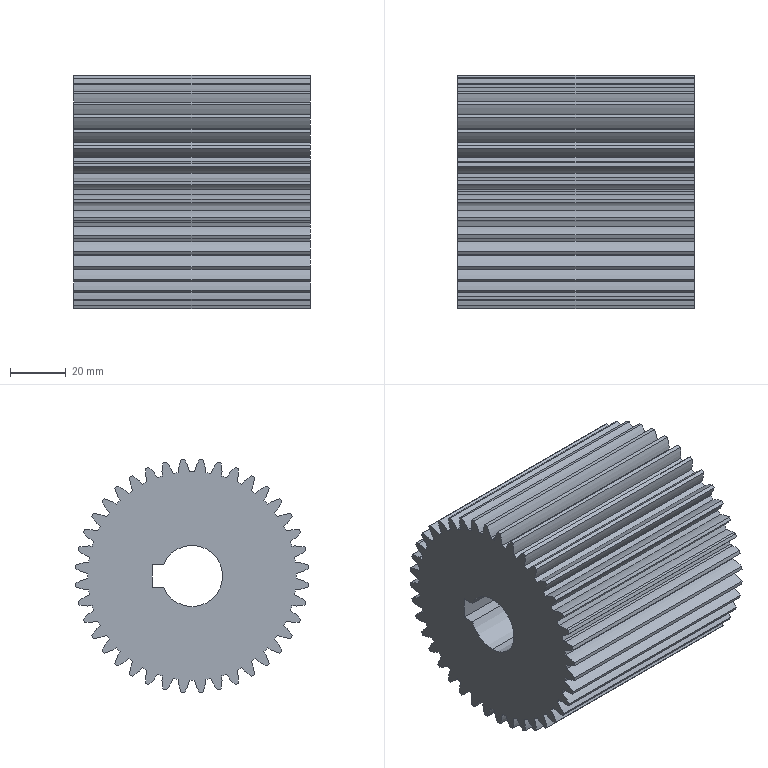Part | SolidWorks | features BaseBody 1 | 1 solid | 173 faces | box 85 x 83.831 x 83.831 mm | volume 385838 mm3 | cylinder 168 | plane 5 | commonest cylinder face diameters 32 x84 74.998 x41 84 x40 22 x3